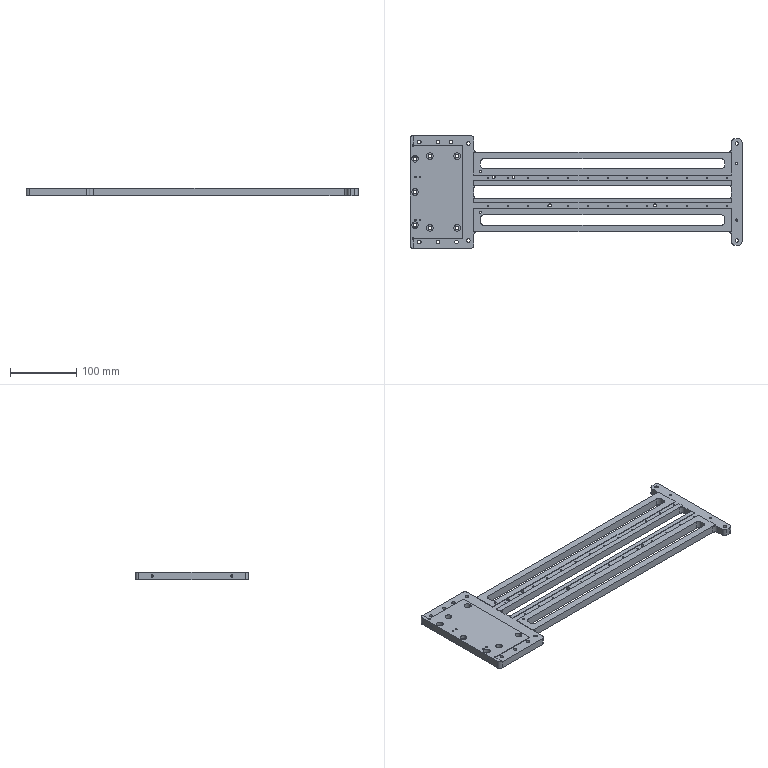Part | STEP file | PN_0005 | 1 solid | 297 faces | box 500 x 170 x 12 mm | volume 536065 mm3 | cylinder 174 | cone 62 | plane 61 | commonest cylinder face diameters 1.6 x52 10 x50 5.5 x26 3.3 x18 2.5 x8 4.2 x8